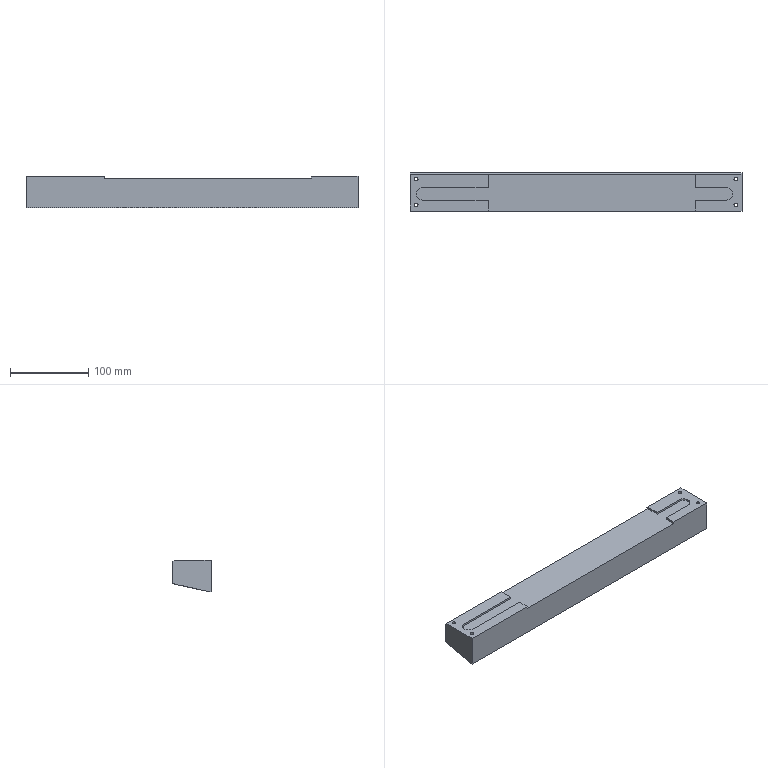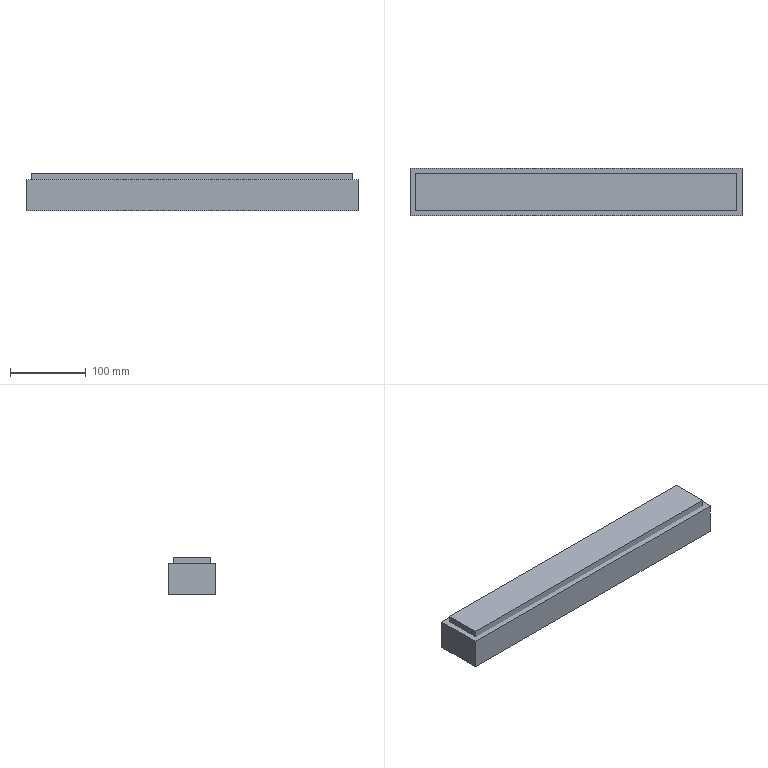CAM job | NX | 3-axis milling, drilling | part box 425 x 49 x 40 mm | stock box 439 x 63 x 50 mm
Tools:
number,name,description,diameter,corner_radius,flute_length,length,flutes
1,D63,Milling Tool-5 Parameters,63.0,0.0,50.0,75.0,2
9,D6A45,Milling Tool-5 Parameters,6.0,0.0,3.0,3.0,2
14,4.5ZT,Drilling Tool,4.5,0.0,35.0,50.0,2
2,D10,Milling Tool-5 Parameters,10.0,0.0,50.0,75.0,2
18,D6R0.5,Milling Tool-5 Parameters,6.0,0.5,50.0,75.0,2
Operations:
program,operation,operation_type,tool,method,geometry_group,spindle_rpm,surface_speed,feed_per_tooth,feed_cut,feed_plunge,cut_length_mm,path_length_mm,cut_time_min,machine_time_min
1-虎钳-430-55-50毛胚,FLOOR_WALL,VolumeBased25DMillingOperation,D63,METHOD,A,6500.0,0.0,0.0,1250.0,100.0,1053.797,1107.797,0.843,0.8484
1-虎钳-430-55-50毛胚,DRILLING,Operation,D6A45,METHOD,A,4000.0,75.0,0.0312,250.0,0.0,16.0,576.283,0.064,0.12
1-虎钳-430-55-50毛胚,DRILLING_COPY,Operation,4.5ZT,METHOD,A,2000.0,20.0,0.05,100.0,0.0,157.408,859.099,1.574,1.644
1-虎钳-430-55-50毛胚,ADAPTIVE_MILLING,CavityMilling,D10,METHOD,A,7000.0,219.0,0.1429,2000.0,1000.0,18281.182,22810.466,9.156,9.608
1-虎钳-430-55-50毛胚,FLOOR_WALL_1,VolumeBased25DMillingOperation,D10,METHOD,A,7000.0,219.0,0.1786,2500.0,1000.0,7157.876,7272.471,2.878,2.89
1-虎钳-430-55-50毛胚,ZLEVEL_PROFILE_COPY_COPY_1,ZLevelMilling,D10,METHOD,A,6500.0,326.0,0.0769,1000.0,1000.0,1976.832,2114.232,1.977,1.991
1-虎钳-430-55-50毛胚,FLOOR_WALL_1_COPY_COPY,VolumeBased25DMillingOperation,D10,METHOD,A,7000.0,219.0,0.0714,1000.0,1000.0,3786.852,4164.967,3.787,3.845
1-虎钳-430-55-50毛胚,ZLEVEL_PROFILE_COPY_1_COPY_COPY_COPY_COPY,ZLevelMilling,D6A45,METHOD,A,7000.0,131.0,0.0714,1000.0,1000.0,838.657,2125.992,0.8387,0.9674
1-虎钳-430-55-50毛胚,ZLEVEL_PROFILE_COPY_1_COPY_COPY_COPY_COPY_COPY,ZLevelMilling,D6A45,METHOD,A,7000.0,131.0,0.0714,1000.0,1000.0,523.986,709.224,0.524,0.5425
2-桥板-430-55-50毛胚,FLOOR_WALL_COPY,VolumeBased25DMillingOperation,D63,METHOD,B,6500.0,0.0,0.0,1250.0,100.0,10117.97,10782.145,8.094,8.161
2-桥板-430-55-50毛胚,ZLEVEL_PROFILE_1,ZLevelMilling,D10,METHOD,B,7000.0,131.0,0.1786,2500.0,1000.0,20982.057,21049.437,8.395,8.402
2-桥板-430-55-50毛胚,ZLEVEL_PROFILE_1_1,ZLevelMilling,D6R0.5,METHOD,B,7000.0,131.0,0.1786,2500.0,1000.0,212399.697,212467.335,84.962,84.969